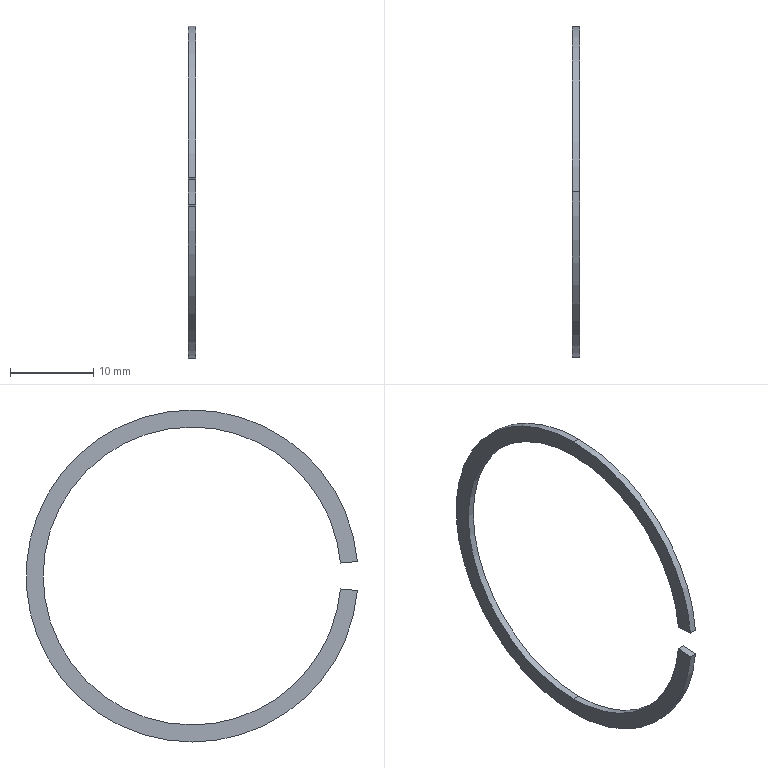Part | STEP file | SB6904ZZNR-Part-1 | 1 solid | 10 faces | box 0.85 x 39.724 x 39.8 mm | volume 200.912 mm3 | cylinder 6 | plane 4 | commonest cylinder face diameters 35.7 x3 39.8 x3
STEP:
#1=CARTESIAN_POINT('',(2.55,0.,-19.9));
#2=VERTEX_POINT('',#1);
#3=CARTESIAN_POINT('',(2.55,0.,19.9));
#4=VERTEX_POINT('',#3);
#5=CARTESIAN_POINT('',(2.55,0.,0.));
#6=DIRECTION('',(1.,0.,0.));
#7=DIRECTION('',(0.,0.,-1.));
#8=AXIS2_PLACEMENT_3D('',#5,#6,#7);
#9=CIRCLE('',#8,19.9);
#10=EDGE_CURVE('',#2,#4,#9,.T.);
#11=ORIENTED_EDGE('',*,*,#10,.F.);
#12=CARTESIAN_POINT('',(1.7,0.,-19.9));
#13=VERTEX_POINT('',#12);
#14=CARTESIAN_POINT('',(2.55,0.,-19.9));
#15=DIRECTION('',(-1.,0.,0.));
#16=VECTOR('',#15,1000.);
#17=LINE('',#14,#16);
#18=EDGE_CURVE('',#2,#13,#17,.T.);
#19=ORIENTED_EDGE('',*,*,#18,.T.);
#20=CARTESIAN_POINT('',(1.7,0.,19.9));
#21=VERTEX_POINT('',#20);
#22=CARTESIAN_POINT('',(1.7,0.,0.));
#23=DIRECTION('',(1.,0.,0.));
#24=DIRECTION('',(0.,0.,-1.));
#25=AXIS2_PLACEMENT_3D('',#22,#23,#24);
#26=CIRCLE('',#25,19.9);
#27=EDGE_CURVE('',#13,#21,#26,.T.);
#28=ORIENTED_EDGE('',*,*,#27,.T.);
#29=CARTESIAN_POINT('',(2.55,0.,19.9));
#30=DIRECTION('',(-1.,0.,0.));
#31=VECTOR('',#30,1000.);
#32=LINE('',#29,#31);
#33=EDGE_CURVE('',#4,#21,#32,.T.);
#34=ORIENTED_EDGE('',*,*,#33,.F.);
#35=EDGE_LOOP('',(#11,#19,#28,#34));
#36=FACE_OUTER_BOUND('',#35,.T.);
#37=CARTESIAN_POINT('',(2.55,0.,0.));
#38=DIRECTION('',(-1.,0.,0.));
#39=DIRECTION('',(0.,0.,1.));
#40=AXIS2_PLACEMENT_3D('',#37,#38,#39);
#41=CYLINDRICAL_SURFACE('',#40,19.9);
#42=ADVANCED_FACE('',(#36),#41,.T.);
#43=CARTESIAN_POINT('',(2.55,-19.824,1.734));
#44=VERTEX_POINT('',#43);
#45=CARTESIAN_POINT('',(2.55,0.,0.));
#46=DIRECTION('',(1.,0.,0.));
#47=DIRECTION('',(0.,0.,-1.));
#48=AXIS2_PLACEMENT_3D('',#45,#46,#47);
#49=CIRCLE('',#48,19.9);
#50=EDGE_CURVE('',#4,#44,#49,.T.);
#51=ORIENTED_EDGE('',*,*,#50,.F.);
#52=ORIENTED_EDGE('',*,*,#33,.T.);
#53=CARTESIAN_POINT('',(1.7,-19.824,1.734));
#54=VERTEX_POINT('',#53);
#55=CARTESIAN_POINT('',(1.7,0.,0.));
#56=DIRECTION('',(1.,0.,0.));
#57=DIRECTION('',(0.,0.,-1.));
#58=AXIS2_PLACEMENT_3D('',#55,#56,#57);
#59=CIRCLE('',#58,19.9);
#60=EDGE_CURVE('',#21,#54,#59,.T.);
#61=ORIENTED_EDGE('',*,*,#60,.T.);
#62=CARTESIAN_POINT('',(2.55,-19.824,1.734));
#63=DIRECTION('',(-1.,0.,0.));
#64=VECTOR('',#63,1000.);
#65=LINE('',#62,#64);
#66=EDGE_CURVE('',#44,#54,#65,.T.);
#67=ORIENTED_EDGE('',*,*,#66,.F.);
#68=EDGE_LOOP('',(#51,#52,#61,#67));
#69=FACE_OUTER_BOUND('',#68,.T.);
#70=CARTESIAN_POINT('',(2.55,0.,0.));
#71=DIRECTION('',(-1.,0.,0.));
#72=DIRECTION('',(0.,0.,1.));
#73=AXIS2_PLACEMENT_3D('',#70,#71,#72);
#74=CYLINDRICAL_SURFACE('',#73,19.9);
#75=ADVANCED_FACE('',(#69),#74,.T.);
#76=CARTESIAN_POINT('',(2.55,0.,-17.85));
#77=VERTEX_POINT('',#76);
#78=CARTESIAN_POINT('',(2.55,-17.782,-1.556));
#79=VERTEX_POINT('',#78);
#80=CARTESIAN_POINT('',(2.55,0.,0.));
#81=DIRECTION('',(-1.,0.,0.));
#82=DIRECTION('',(0.,0.,-1.));
#83=AXIS2_PLACEMENT_3D('',#80,#81,#82);
#84=CIRCLE('',#83,17.85);
#85=EDGE_CURVE('',#77,#79,#84,.T.);
#86=ORIENTED_EDGE('',*,*,#85,.F.);
#87=CARTESIAN_POINT('',(1.7,0.,-17.85));
#88=VERTEX_POINT('',#87);
#89=CARTESIAN_POINT('',(2.55,0.,-17.85));
#90=DIRECTION('',(-1.,0.,0.));
#91=VECTOR('',#90,1000.);
#92=LINE('',#89,#91);
#93=EDGE_CURVE('',#77,#88,#92,.T.);
#94=ORIENTED_EDGE('',*,*,#93,.T.);
#95=CARTESIAN_POINT('',(1.7,-17.782,-1.556));
#96=VERTEX_POINT('',#95);
#97=CARTESIAN_POINT('',(1.7,0.,0.));
#98=DIRECTION('',(-1.,0.,0.));
#99=DIRECTION('',(0.,0.,-1.));
#100=AXIS2_PLACEMENT_3D('',#97,#98,#99);
#101=CIRCLE('',#100,17.85);
#102=EDGE_CURVE('',#88,#96,#101,.T.);
#103=ORIENTED_EDGE('',*,*,#102,.T.);
#104=CARTESIAN_POINT('',(2.55,-17.782,-1.556));
#105=DIRECTION('',(-1.,0.,0.));
#106=VECTOR('',#105,1000.);
#107=LINE('',#104,#106);
#108=EDGE_CURVE('',#79,#96,#107,.T.);
#109=ORIENTED_EDGE('',*,*,#108,.F.);
#110=EDGE_LOOP('',(#86,#94,#103,#109));
#111=FACE_OUTER_BOUND('',#110,.T.);
#112=CARTESIAN_POINT('',(2.55,0.,0.));
#113=DIRECTION('',(-1.,0.,0.));
#114=DIRECTION('',(0.,0.,1.));
#115=AXIS2_PLACEMENT_3D('',#112,#113,#114);
#116=CYLINDRICAL_SURFACE('',#115,17.85);
#117=ADVANCED_FACE('',(#111),#116,.F.);
#118=ORIENTED_EDGE('',*,*,#93,.F.);
#119=CARTESIAN_POINT('',(2.55,0.,17.85));
#120=VERTEX_POINT('',#119);
#121=CARTESIAN_POINT('',(2.55,0.,0.));
#122=DIRECTION('',(-1.,0.,0.));
#123=DIRECTION('',(0.,0.,-1.));
#124=AXIS2_PLACEMENT_3D('',#121,#122,#123);
#125=CIRCLE('',#124,17.85);
#126=EDGE_CURVE('',#120,#77,#125,.T.);
#127=ORIENTED_EDGE('',*,*,#126,.F.);
#128=CARTESIAN_POINT('',(1.7,0.,17.85));
#129=VERTEX_POINT('',#128);
#130=CARTESIAN_POINT('',(2.55,0.,17.85));
#131=DIRECTION('',(-1.,0.,0.));
#132=VECTOR('',#131,1000.);
#133=LINE('',#130,#132);
#134=EDGE_CURVE('',#120,#129,#133,.T.);
#135=ORIENTED_EDGE('',*,*,#134,.T.);
#136=CARTESIAN_POINT('',(1.7,0.,0.));
#137=DIRECTION('',(-1.,0.,0.));
#138=DIRECTION('',(0.,0.,-1.));
#139=AXIS2_PLACEMENT_3D('',#136,#137,#138);
#140=CIRCLE('',#139,17.85);
#141=EDGE_CURVE('',#129,#88,#140,.T.);
#142=ORIENTED_EDGE('',*,*,#141,.T.);
#143=EDGE_LOOP('',(#118,#127,#135,#142));
#144=FACE_OUTER_BOUND('',#143,.T.);
#145=CARTESIAN_POINT('',(2.55,0.,0.));
#146=DIRECTION('',(-1.,0.,0.));
#147=DIRECTION('',(0.,0.,1.));
#148=AXIS2_PLACEMENT_3D('',#145,#146,#147);
#149=CYLINDRICAL_SURFACE('',#148,17.85);
#150=ADVANCED_FACE('',(#144),#149,.F.);
#151=ORIENTED_EDGE('',*,*,#134,.F.);
#152=CARTESIAN_POINT('',(2.55,-17.782,1.556));
#153=VERTEX_POINT('',#152);
#154=CARTESIAN_POINT('',(2.55,0.,0.));
#155=DIRECTION('',(-1.,0.,0.));
#156=DIRECTION('',(0.,0.,-1.));
#157=AXIS2_PLACEMENT_3D('',#154,#155,#156);
#158=CIRCLE('',#157,17.85);
#159=EDGE_CURVE('',#153,#120,#158,.T.);
#160=ORIENTED_EDGE('',*,*,#159,.F.);
#161=CARTESIAN_POINT('',(1.7,-17.782,1.556));
#162=VERTEX_POINT('',#161);
#163=CARTESIAN_POINT('',(2.55,-17.782,1.556));
#164=DIRECTION('',(-1.,0.,0.));
#165=VECTOR('',#164,1000.);
#166=LINE('',#163,#165);
#167=EDGE_CURVE('',#153,#162,#166,.T.);
#168=ORIENTED_EDGE('',*,*,#167,.T.);
#169=CARTESIAN_POINT('',(1.7,0.,0.));
#170=DIRECTION('',(-1.,0.,0.));
#171=DIRECTION('',(0.,0.,-1.));
#172=AXIS2_PLACEMENT_3D('',#169,#170,#171);
#173=CIRCLE('',#172,17.85);
#174=EDGE_CURVE('',#162,#129,#173,.T.);
#175=ORIENTED_EDGE('',*,*,#174,.T.);
#176=EDGE_LOOP('',(#151,#160,#168,#175));
#177=FACE_OUTER_BOUND('',#176,.T.);
#178=CARTESIAN_POINT('',(2.55,0.,0.));
#179=DIRECTION('',(-1.,0.,0.));
#180=DIRECTION('',(0.,0.,1.));
#181=AXIS2_PLACEMENT_3D('',#178,#179,#180);
#182=CYLINDRICAL_SURFACE('',#181,17.85);
#183=ADVANCED_FACE('',(#177),#182,.F.);
#184=CARTESIAN_POINT('',(1.7,-19.824,-1.734));
#185=VERTEX_POINT('',#184);
#186=CARTESIAN_POINT('',(1.7,-17.782,-1.556));
#187=DIRECTION('',(0.,-0.9962,-0.08716));
#188=VECTOR('',#187,1000.);
#189=LINE('',#186,#188);
#190=EDGE_CURVE('',#96,#185,#189,.T.);
#191=ORIENTED_EDGE('',*,*,#190,.T.);
#192=CARTESIAN_POINT('',(2.55,-19.824,-1.734));
#193=VERTEX_POINT('',#192);
#194=CARTESIAN_POINT('',(2.55,-19.824,-1.734));
#195=DIRECTION('',(-1.,0.,0.));
#196=VECTOR('',#195,1000.);
#197=LINE('',#194,#196);
#198=EDGE_CURVE('',#193,#185,#197,.T.);
#199=ORIENTED_EDGE('',*,*,#198,.F.);
#200=CARTESIAN_POINT('',(2.55,-17.782,-1.556));
#201=DIRECTION('',(0.,-0.9962,-0.08716));
#202=VECTOR('',#201,1000.);
#203=LINE('',#200,#202);
#204=EDGE_CURVE('',#79,#193,#203,.T.);
#205=ORIENTED_EDGE('',*,*,#204,.F.);
#206=ORIENTED_EDGE('',*,*,#108,.T.);
#207=EDGE_LOOP('',(#191,#199,#205,#206));
#208=FACE_OUTER_BOUND('',#207,.T.);
#209=CARTESIAN_POINT('',(2.55,-17.782,-1.556));
#210=DIRECTION('',(0.,0.08716,-0.9962));
#211=DIRECTION('',(0.,0.9962,0.08716));
#212=AXIS2_PLACEMENT_3D('',#209,#210,#211);
#213=PLANE('',#212);
#214=ADVANCED_FACE('',(#208),#213,.F.);
#215=ORIENTED_EDGE('',*,*,#18,.F.);
#216=CARTESIAN_POINT('',(2.55,0.,0.));
#217=DIRECTION('',(1.,0.,0.));
#218=DIRECTION('',(0.,0.,-1.));
#219=AXIS2_PLACEMENT_3D('',#216,#217,#218);
#220=CIRCLE('',#219,19.9);
#221=EDGE_CURVE('',#193,#2,#220,.T.);
#222=ORIENTED_EDGE('',*,*,#221,.F.);
#223=ORIENTED_EDGE('',*,*,#198,.T.);
#224=CARTESIAN_POINT('',(1.7,0.,0.));
#225=DIRECTION('',(1.,0.,0.));
#226=DIRECTION('',(0.,0.,-1.));
#227=AXIS2_PLACEMENT_3D('',#224,#225,#226);
#228=CIRCLE('',#227,19.9);
#229=EDGE_CURVE('',#185,#13,#228,.T.);
#230=ORIENTED_EDGE('',*,*,#229,.T.);
#231=EDGE_LOOP('',(#215,#222,#223,#230));
#232=FACE_OUTER_BOUND('',#231,.T.);
#233=CARTESIAN_POINT('',(2.55,0.,0.));
#234=DIRECTION('',(-1.,0.,0.));
#235=DIRECTION('',(0.,0.,1.));
#236=AXIS2_PLACEMENT_3D('',#233,#234,#235);
#237=CYLINDRICAL_SURFACE('',#236,19.9);
#238=ADVANCED_FACE('',(#232),#237,.T.);
#239=CARTESIAN_POINT('',(1.7,-17.782,1.556));
#240=DIRECTION('',(0.,0.9962,-0.08716));
#241=VECTOR('',#240,1000.);
#242=LINE('',#239,#241);
#243=EDGE_CURVE('',#54,#162,#242,.T.);
#244=ORIENTED_EDGE('',*,*,#243,.T.);
#245=ORIENTED_EDGE('',*,*,#167,.F.);
#246=CARTESIAN_POINT('',(2.55,-17.782,1.556));
#247=DIRECTION('',(0.,0.9962,-0.08716));
#248=VECTOR('',#247,1000.);
#249=LINE('',#246,#248);
#250=EDGE_CURVE('',#44,#153,#249,.T.);
#251=ORIENTED_EDGE('',*,*,#250,.F.);
#252=ORIENTED_EDGE('',*,*,#66,.T.);
#253=EDGE_LOOP('',(#244,#245,#251,#252));
#254=FACE_OUTER_BOUND('',#253,.T.);
#255=CARTESIAN_POINT('',(2.55,-17.782,1.556));
#256=DIRECTION('',(0.,0.08716,0.9962));
#257=DIRECTION('',(0.,-0.9962,0.08716));
#258=AXIS2_PLACEMENT_3D('',#255,#256,#257);
#259=PLANE('',#258);
#260=ADVANCED_FACE('',(#254),#259,.F.);
#261=ORIENTED_EDGE('',*,*,#159,.T.);
#262=ORIENTED_EDGE('',*,*,#126,.T.);
#263=ORIENTED_EDGE('',*,*,#85,.T.);
#264=ORIENTED_EDGE('',*,*,#204,.T.);
#265=ORIENTED_EDGE('',*,*,#221,.T.);
#266=ORIENTED_EDGE('',*,*,#10,.T.);
#267=ORIENTED_EDGE('',*,*,#50,.T.);
#268=ORIENTED_EDGE('',*,*,#250,.T.);
#269=EDGE_LOOP('',(#261,#262,#263,#264,#265,#266,#267,#268));
#270=FACE_OUTER_BOUND('',#269,.T.);
#271=CARTESIAN_POINT('',(2.55,0.,0.));
#272=DIRECTION('',(1.,0.,0.));
#273=DIRECTION('',(0.,0.,-1.));
#274=AXIS2_PLACEMENT_3D('',#271,#272,#273);
#275=PLANE('',#274);
#276=ADVANCED_FACE('',(#270),#275,.T.);
#277=ORIENTED_EDGE('',*,*,#174,.F.);
#278=ORIENTED_EDGE('',*,*,#243,.F.);
#279=ORIENTED_EDGE('',*,*,#60,.F.);
#280=ORIENTED_EDGE('',*,*,#27,.F.);
#281=ORIENTED_EDGE('',*,*,#229,.F.);
#282=ORIENTED_EDGE('',*,*,#190,.F.);
#283=ORIENTED_EDGE('',*,*,#102,.F.);
#284=ORIENTED_EDGE('',*,*,#141,.F.);
#285=EDGE_LOOP('',(#277,#278,#279,#280,#281,#282,#283,#284));
#286=FACE_OUTER_BOUND('',#285,.T.);
#287=CARTESIAN_POINT('',(1.7,0.,0.));
#288=DIRECTION('',(1.,0.,0.));
#289=DIRECTION('',(0.,0.,-1.));
#290=AXIS2_PLACEMENT_3D('',#287,#288,#289);
#291=PLANE('',#290);
#292=ADVANCED_FACE('',(#286),#291,.F.);
#293=CLOSED_SHELL('',(#42,#75,#117,#150,#183,#214,#238,#260,#276,#292));
#294=MANIFOLD_SOLID_BREP('',#293);
#295=CARTESIAN_POINT('',(0.,0.,0.));
#296=DIRECTION('',(0.,0.,1.));
#297=DIRECTION('',(1.,0.,0.));
#298=AXIS2_PLACEMENT_3D('',#295,#296,#297);
#299=(LENGTH_UNIT()NAMED_UNIT(*)SI_UNIT(.MILLI.,.METRE.));
#300=UNCERTAINTY_MEASURE_WITH_UNIT(LENGTH_MEASURE(0.00001),#299,'','');
#301=(NAMED_UNIT(*)PLANE_ANGLE_UNIT()SI_UNIT($,.RADIAN.));
#302=(NAMED_UNIT(*)SI_UNIT($,.STERADIAN.)SOLID_ANGLE_UNIT());
#303=(GEOMETRIC_REPRESENTATION_CONTEXT(3)GLOBAL_UNCERTAINTY_ASSIGNED_CONTEXT((#300))GLOBAL_UNIT_ASSIGNED_CONTEXT((#299,#301,#302))REPRESENTATION_CONTEXT('',''));
#304=ADVANCED_BREP_SHAPE_REPRESENTATION('',(#294,#298),#303);